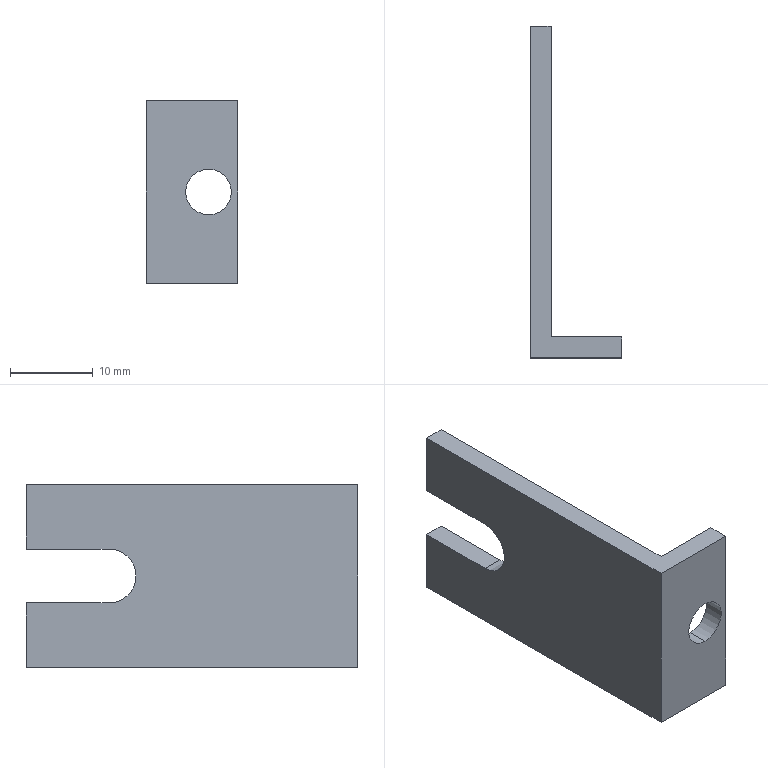Part | STEP file | slingshot track fixed block | 1 solid | 14 faces | box 11 x 40 x 22 mm | volume 2404 mm3 | plane 11 | cylinder 3 | commonest cylinder face diameters 5.5 x2 6.5 x1
STEP:
#1=CARTESIAN_POINT('',(0.,0.,0.));
#2=DIRECTION('',(0.,0.,1.));
#3=DIRECTION('',(1.,0.,0.));
#4=AXIS2_PLACEMENT_3D('',#1,#2,#3);
#5=CARTESIAN_POINT('',(7.5,0.,13.75));
#6=VERTEX_POINT('',#5);
#7=CARTESIAN_POINT('',(7.5,2.5,13.75));
#8=VERTEX_POINT('',#7);
#9=CARTESIAN_POINT('',(7.5,-19.5,13.75));
#10=DIRECTION('',(0.,1.,0.));
#11=VECTOR('',#10,1.);
#12=LINE('',#9,#11);
#13=CARTESIAN_POINT('',(7.5,-19.5,11.));
#14=DIRECTION('',(0.,1.,0.));
#15=DIRECTION('',(0.,0.,1.));
#16=AXIS2_PLACEMENT_3D('',#13,#14,#15);
#17=CYLINDRICAL_SURFACE('',#16,2.75);
#18=CARTESIAN_POINT('',(6.283,0.));
#19=DIRECTION('',(0.,1.));
#20=VECTOR('',#19,1.);
#21=LINE('',#18,#20);
#22=(GEOMETRIC_REPRESENTATION_CONTEXT(2)PARAMETRIC_REPRESENTATION_CONTEXT()REPRESENTATION_CONTEXT('',''));
#23=DEFINITIONAL_REPRESENTATION('',(#21),#22);
#24=PCURVE('',#17,#23);
#25=CARTESIAN_POINT('',(7.5,-19.5,11.));
#26=DIRECTION('',(0.,1.,0.));
#27=DIRECTION('',(0.,0.,1.));
#28=AXIS2_PLACEMENT_3D('',#25,#26,#27);
#29=CYLINDRICAL_SURFACE('',#28,2.75);
#30=CARTESIAN_POINT('',(0.,0.));
#31=DIRECTION('',(0.,1.));
#32=VECTOR('',#31,1.);
#33=LINE('',#30,#32);
#34=(GEOMETRIC_REPRESENTATION_CONTEXT(2)PARAMETRIC_REPRESENTATION_CONTEXT()REPRESENTATION_CONTEXT('',''));
#35=DEFINITIONAL_REPRESENTATION('',(#33),#34);
#36=PCURVE('',#29,#35);
#37=SURFACE_CURVE('',#12,(#24,#36),.PCURVE_S1.);
#38=EDGE_CURVE('',#6,#8,#37,.T.);
#39=ORIENTED_EDGE('',*,*,#38,.T.);
#40=CARTESIAN_POINT('',(7.5,2.5,8.25));
#41=VERTEX_POINT('',#40);
#42=CARTESIAN_POINT('',(7.5,2.5,11.));
#43=DIRECTION('',(0.,1.,0.));
#44=DIRECTION('',(0.,0.,1.));
#45=AXIS2_PLACEMENT_3D('',#42,#43,#44);
#46=CIRCLE('',#45,2.75);
#47=CARTESIAN_POINT('',(0.,22.));
#48=DIRECTION('',(1.,0.));
#49=VECTOR('',#48,1.);
#50=LINE('',#47,#49);
#51=(GEOMETRIC_REPRESENTATION_CONTEXT(2)PARAMETRIC_REPRESENTATION_CONTEXT()REPRESENTATION_CONTEXT('',''));
#52=DEFINITIONAL_REPRESENTATION('',(#50),#51);
#53=PCURVE('',#17,#52);
#54=CARTESIAN_POINT('',(2.5,2.5,22.));
#55=DIRECTION('',(0.,-1.,0.));
#56=DIRECTION('',(0.,0.,-1.));
#57=AXIS2_PLACEMENT_3D('',#54,#55,#56);
#58=PLANE('',#57);
#59=CARTESIAN_POINT('',(8.25,5.));
#60=CARTESIAN_POINT('',(8.25,9.763));
#61=CARTESIAN_POINT('',(12.375,7.382));
#62=CARTESIAN_POINT('',(16.5,5.));
#63=CARTESIAN_POINT('',(12.375,2.618));
#64=CARTESIAN_POINT('',(8.25,0.2369));
#65=CARTESIAN_POINT('',(8.25,5.));
#66=(BOUNDED_CURVE()B_SPLINE_CURVE(2,(#59,#60,#61,#62,#63,#64,#65),.UNSPECIFIED.,.T.,.F.)B_SPLINE_CURVE_WITH_KNOTS((1,2,2,2,2,1),(-2.094,0.,2.094,4.189,6.283,8.378),.UNSPECIFIED.)CURVE()GEOMETRIC_REPRESENTATION_ITEM()RATIONAL_B_SPLINE_CURVE((1.,0.5,1.,0.5,1.,0.5,1.))REPRESENTATION_ITEM(''));
#67=(GEOMETRIC_REPRESENTATION_CONTEXT(2)PARAMETRIC_REPRESENTATION_CONTEXT()REPRESENTATION_CONTEXT('',''));
#68=DEFINITIONAL_REPRESENTATION('',(#66),#67);
#69=PCURVE('',#58,#68);
#70=SURFACE_CURVE('',#46,(#53,#69),.PCURVE_S1.);
#71=EDGE_CURVE('',#41,#8,#70,.T.);
#72=ORIENTED_EDGE('',*,*,#71,.F.);
#73=CARTESIAN_POINT('',(7.5,0.,8.25));
#74=VERTEX_POINT('',#73);
#75=CARTESIAN_POINT('',(7.5,-19.5,8.25));
#76=DIRECTION('',(0.,1.,0.));
#77=VECTOR('',#76,1.);
#78=LINE('',#75,#77);
#79=CARTESIAN_POINT('',(3.142,0.));
#80=DIRECTION('',(0.,1.));
#81=VECTOR('',#80,1.);
#82=LINE('',#79,#81);
#83=(GEOMETRIC_REPRESENTATION_CONTEXT(2)PARAMETRIC_REPRESENTATION_CONTEXT()REPRESENTATION_CONTEXT('',''));
#84=DEFINITIONAL_REPRESENTATION('',(#82),#83);
#85=PCURVE('',#17,#84);
#86=CARTESIAN_POINT('',(3.142,0.));
#87=DIRECTION('',(0.,1.));
#88=VECTOR('',#87,1.);
#89=LINE('',#86,#88);
#90=(GEOMETRIC_REPRESENTATION_CONTEXT(2)PARAMETRIC_REPRESENTATION_CONTEXT()REPRESENTATION_CONTEXT('',''));
#91=DEFINITIONAL_REPRESENTATION('',(#89),#90);
#92=PCURVE('',#29,#91);
#93=SURFACE_CURVE('',#78,(#85,#92),.PCURVE_S1.);
#94=EDGE_CURVE('',#74,#41,#93,.T.);
#95=ORIENTED_EDGE('',*,*,#94,.F.);
#96=CARTESIAN_POINT('',(7.5,0.,11.));
#97=DIRECTION('',(0.,1.,0.));
#98=DIRECTION('',(0.,0.,1.));
#99=AXIS2_PLACEMENT_3D('',#96,#97,#98);
#100=CIRCLE('',#99,2.75);
#101=CARTESIAN_POINT('',(0.,19.5));
#102=DIRECTION('',(1.,0.));
#103=VECTOR('',#102,1.);
#104=LINE('',#101,#103);
#105=(GEOMETRIC_REPRESENTATION_CONTEXT(2)PARAMETRIC_REPRESENTATION_CONTEXT()REPRESENTATION_CONTEXT('',''));
#106=DEFINITIONAL_REPRESENTATION('',(#104),#105);
#107=PCURVE('',#17,#106);
#108=CARTESIAN_POINT('',(0.,0.,22.));
#109=DIRECTION('',(0.,1.,0.));
#110=DIRECTION('',(0.,0.,1.));
#111=AXIS2_PLACEMENT_3D('',#108,#109,#110);
#112=PLANE('',#111);
#113=CARTESIAN_POINT('',(-11.,7.5));
#114=DIRECTION('',(1.,0.));
#115=AXIS2_PLACEMENT_2D('',#113,#114);
#116=CIRCLE('',#115,2.75);
#117=(GEOMETRIC_REPRESENTATION_CONTEXT(2)PARAMETRIC_REPRESENTATION_CONTEXT()REPRESENTATION_CONTEXT('',''));
#118=DEFINITIONAL_REPRESENTATION('',(#116),#117);
#119=PCURVE('',#112,#118);
#120=SURFACE_CURVE('',#100,(#107,#119),.PCURVE_S1.);
#121=EDGE_CURVE('',#74,#6,#120,.T.);
#122=ORIENTED_EDGE('',*,*,#121,.T.);
#123=EDGE_LOOP('',(#39,#72,#95,#122));
#124=FACE_BOUND('',#123,.F.);
#125=ADVANCED_FACE('',(#124),#17,.F.);
#126=CARTESIAN_POINT('',(0.,40.,7.75));
#127=VERTEX_POINT('',#126);
#128=CARTESIAN_POINT('',(0.,40.,0.));
#129=VERTEX_POINT('',#128);
#130=CARTESIAN_POINT('',(0.,40.,22.));
#131=DIRECTION('',(0.,0.,-1.));
#132=VECTOR('',#131,1.);
#133=LINE('',#130,#132);
#134=CARTESIAN_POINT('',(0.,40.,22.));
#135=DIRECTION('',(0.,-1.,0.));
#136=DIRECTION('',(0.,0.,-1.));
#137=AXIS2_PLACEMENT_3D('',#134,#135,#136);
#138=PLANE('',#137);
#139=CARTESIAN_POINT('',(0.,0.));
#140=DIRECTION('',(1.,0.));
#141=VECTOR('',#140,1.);
#142=LINE('',#139,#141);
#143=(GEOMETRIC_REPRESENTATION_CONTEXT(2)PARAMETRIC_REPRESENTATION_CONTEXT()REPRESENTATION_CONTEXT('',''));
#144=DEFINITIONAL_REPRESENTATION('',(#142),#143);
#145=PCURVE('',#138,#144);
#146=CARTESIAN_POINT('',(0.,0.,22.));
#147=DIRECTION('',(1.,0.,0.));
#148=DIRECTION('',(0.,0.,-1.));
#149=AXIS2_PLACEMENT_3D('',#146,#147,#148);
#150=PLANE('',#149);
#151=CARTESIAN_POINT('',(0.,40.));
#152=DIRECTION('',(1.,0.));
#153=VECTOR('',#152,1.);
#154=LINE('',#151,#153);
#155=(GEOMETRIC_REPRESENTATION_CONTEXT(2)PARAMETRIC_REPRESENTATION_CONTEXT()REPRESENTATION_CONTEXT('',''));
#156=DEFINITIONAL_REPRESENTATION('',(#154),#155);
#157=PCURVE('',#150,#156);
#158=SURFACE_CURVE('',#133,(#145,#157),.PCURVE_S1.);
#159=EDGE_CURVE('',#127,#129,#158,.T.);
#160=ORIENTED_EDGE('',*,*,#159,.F.);
#161=CARTESIAN_POINT('',(2.5,40.,7.75));
#162=VERTEX_POINT('',#161);
#163=CARTESIAN_POINT('',(0.,40.,7.75));
#164=DIRECTION('',(1.,0.,0.));
#165=VECTOR('',#164,1.);
#166=LINE('',#163,#165);
#167=CARTESIAN_POINT('',(14.25,0.));
#168=DIRECTION('',(0.,1.));
#169=VECTOR('',#168,1.);
#170=LINE('',#167,#169);
#171=(GEOMETRIC_REPRESENTATION_CONTEXT(2)PARAMETRIC_REPRESENTATION_CONTEXT()REPRESENTATION_CONTEXT('',''));
#172=DEFINITIONAL_REPRESENTATION('',(#170),#171);
#173=PCURVE('',#138,#172);
#174=CARTESIAN_POINT('',(22.,30.,7.75));
#175=DIRECTION('',(0.,0.,-1.));
#176=DIRECTION('',(-1.,0.,0.));
#177=AXIS2_PLACEMENT_3D('',#174,#175,#176);
#178=PLANE('',#177);
#179=CARTESIAN_POINT('',(22.,10.));
#180=DIRECTION('',(-1.,0.));
#181=VECTOR('',#180,1.);
#182=LINE('',#179,#181);
#183=(GEOMETRIC_REPRESENTATION_CONTEXT(2)PARAMETRIC_REPRESENTATION_CONTEXT()REPRESENTATION_CONTEXT('',''));
#184=DEFINITIONAL_REPRESENTATION('',(#182),#183);
#185=PCURVE('',#178,#184);
#186=SURFACE_CURVE('',#166,(#173,#185),.PCURVE_S1.);
#187=EDGE_CURVE('',#127,#162,#186,.T.);
#188=ORIENTED_EDGE('',*,*,#187,.T.);
#189=CARTESIAN_POINT('',(2.5,40.,0.));
#190=VERTEX_POINT('',#189);
#191=CARTESIAN_POINT('',(2.5,40.,22.));
#192=DIRECTION('',(0.,0.,-1.));
#193=VECTOR('',#192,1.);
#194=LINE('',#191,#193);
#195=CARTESIAN_POINT('',(0.,2.5));
#196=DIRECTION('',(1.,0.));
#197=VECTOR('',#196,1.);
#198=LINE('',#195,#197);
#199=(GEOMETRIC_REPRESENTATION_CONTEXT(2)PARAMETRIC_REPRESENTATION_CONTEXT()REPRESENTATION_CONTEXT('',''));
#200=DEFINITIONAL_REPRESENTATION('',(#198),#199);
#201=PCURVE('',#138,#200);
#202=CARTESIAN_POINT('',(2.5,2.5,22.));
#203=DIRECTION('',(-1.,0.,0.));
#204=DIRECTION('',(0.,-1.,0.));
#205=AXIS2_PLACEMENT_3D('',#202,#203,#204);
#206=PLANE('',#205);
#207=CARTESIAN_POINT('',(-37.5,0.));
#208=DIRECTION('',(0.,-1.));
#209=VECTOR('',#208,1.);
#210=LINE('',#207,#209);
#211=(GEOMETRIC_REPRESENTATION_CONTEXT(2)PARAMETRIC_REPRESENTATION_CONTEXT()REPRESENTATION_CONTEXT('',''));
#212=DEFINITIONAL_REPRESENTATION('',(#210),#211);
#213=PCURVE('',#206,#212);
#214=SURFACE_CURVE('',#194,(#201,#213),.PCURVE_S1.);
#215=EDGE_CURVE('',#162,#190,#214,.T.);
#216=ORIENTED_EDGE('',*,*,#215,.T.);
#217=CARTESIAN_POINT('',(0.,40.,0.));
#218=DIRECTION('',(-1.,0.,0.));
#219=VECTOR('',#218,1.);
#220=LINE('',#217,#219);
#221=CARTESIAN_POINT('',(22.,0.));
#222=DIRECTION('',(0.,-1.));
#223=VECTOR('',#222,1.);
#224=LINE('',#221,#223);
#225=(GEOMETRIC_REPRESENTATION_CONTEXT(2)PARAMETRIC_REPRESENTATION_CONTEXT()REPRESENTATION_CONTEXT('',''));
#226=DEFINITIONAL_REPRESENTATION('',(#224),#225);
#227=PCURVE('',#138,#226);
#228=CARTESIAN_POINT('',(0.,40.,0.));
#229=DIRECTION('',(0.,0.,-1.));
#230=DIRECTION('',(-1.,0.,0.));
#231=AXIS2_PLACEMENT_3D('',#228,#229,#230);
#232=PLANE('',#231);
#233=CARTESIAN_POINT('',(0.,0.));
#234=DIRECTION('',(1.,0.));
#235=VECTOR('',#234,1.);
#236=LINE('',#233,#235);
#237=(GEOMETRIC_REPRESENTATION_CONTEXT(2)PARAMETRIC_REPRESENTATION_CONTEXT()REPRESENTATION_CONTEXT('',''));
#238=DEFINITIONAL_REPRESENTATION('',(#236),#237);
#239=PCURVE('',#232,#238);
#240=SURFACE_CURVE('',#220,(#227,#239),.PCURVE_S1.);
#241=EDGE_CURVE('',#190,#129,#240,.T.);
#242=ORIENTED_EDGE('',*,*,#241,.T.);
#243=EDGE_LOOP('',(#160,#188,#216,#242));
#244=FACE_BOUND('',#243,.T.);
#245=ADVANCED_FACE('',(#244),#138,.F.);
#246=CARTESIAN_POINT('',(0.,30.,7.75));
#247=VERTEX_POINT('',#246);
#248=CARTESIAN_POINT('',(0.,30.,14.25));
#249=VERTEX_POINT('',#248);
#250=CARTESIAN_POINT('',(0.,30.,11.));
#251=DIRECTION('',(-1.,0.,0.));
#252=DIRECTION('',(0.,0.,1.));
#253=AXIS2_PLACEMENT_3D('',#250,#251,#252);
#254=CIRCLE('',#253,3.25);
#255=CARTESIAN_POINT('',(7.75,30.));
#256=CARTESIAN_POINT('',(7.75,35.629));
#257=CARTESIAN_POINT('',(12.625,32.815));
#258=CARTESIAN_POINT('',(17.5,30.));
#259=CARTESIAN_POINT('',(12.625,27.185));
#260=CARTESIAN_POINT('',(7.75,24.371));
#261=CARTESIAN_POINT('',(7.75,30.));
#262=(BOUNDED_CURVE()B_SPLINE_CURVE(2,(#255,#256,#257,#258,#259,#260,#261),.UNSPECIFIED.,.T.,.F.)B_SPLINE_CURVE_WITH_KNOTS((1,2,2,2,2,1),(-2.094,0.,2.094,4.189,6.283,8.378),.UNSPECIFIED.)CURVE()GEOMETRIC_REPRESENTATION_ITEM()RATIONAL_B_SPLINE_CURVE((1.,0.5,1.,0.5,1.,0.5,1.))REPRESENTATION_ITEM(''));
#263=(GEOMETRIC_REPRESENTATION_CONTEXT(2)PARAMETRIC_REPRESENTATION_CONTEXT()REPRESENTATION_CONTEXT('',''));
#264=DEFINITIONAL_REPRESENTATION('',(#262),#263);
#265=PCURVE('',#150,#264);
#266=CARTESIAN_POINT('',(22.,30.,11.));
#267=DIRECTION('',(-1.,0.,0.));
#268=DIRECTION('',(0.,0.,1.));
#269=AXIS2_PLACEMENT_3D('',#266,#267,#268);
#270=CYLINDRICAL_SURFACE('',#269,3.25);
#271=CARTESIAN_POINT('',(0.,22.));
#272=DIRECTION('',(1.,0.));
#273=VECTOR('',#272,1.);
#274=LINE('',#271,#273);
#275=(GEOMETRIC_REPRESENTATION_CONTEXT(2)PARAMETRIC_REPRESENTATION_CONTEXT()REPRESENTATION_CONTEXT('',''));
#276=DEFINITIONAL_REPRESENTATION('',(#274),#275);
#277=PCURVE('',#270,#276);
#278=SURFACE_CURVE('',#254,(#265,#277),.PCURVE_S1.);
#279=EDGE_CURVE('',#247,#249,#278,.T.);
#280=ORIENTED_EDGE('',*,*,#279,.F.);
#281=CARTESIAN_POINT('',(0.,30.,7.75));
#282=DIRECTION('',(0.,-1.,0.));
#283=VECTOR('',#282,1.);
#284=LINE('',#281,#283);
#285=CARTESIAN_POINT('',(14.25,30.));
#286=DIRECTION('',(0.,-1.));
#287=VECTOR('',#286,1.);
#288=LINE('',#285,#287);
#289=(GEOMETRIC_REPRESENTATION_CONTEXT(2)PARAMETRIC_REPRESENTATION_CONTEXT()REPRESENTATION_CONTEXT('',''));
#290=DEFINITIONAL_REPRESENTATION('',(#288),#289);
#291=PCURVE('',#150,#290);
#292=CARTESIAN_POINT('',(22.,0.));
#293=DIRECTION('',(0.,-1.));
#294=VECTOR('',#293,1.);
#295=LINE('',#292,#294);
#296=(GEOMETRIC_REPRESENTATION_CONTEXT(2)PARAMETRIC_REPRESENTATION_CONTEXT()REPRESENTATION_CONTEXT('',''));
#297=DEFINITIONAL_REPRESENTATION('',(#295),#296);
#298=PCURVE('',#178,#297);
#299=SURFACE_CURVE('',#284,(#291,#298),.PCURVE_S1.);
#300=EDGE_CURVE('',#127,#247,#299,.T.);
#301=ORIENTED_EDGE('',*,*,#300,.F.);
#302=ORIENTED_EDGE('',*,*,#159,.T.);
#303=CARTESIAN_POINT('',(0.,0.,0.));
#304=VERTEX_POINT('',#303);
#305=CARTESIAN_POINT('',(0.,0.,0.));
#306=DIRECTION('',(0.,-1.,0.));
#307=VECTOR('',#306,1.);
#308=LINE('',#305,#307);
#309=CARTESIAN_POINT('',(22.,0.));
#310=DIRECTION('',(0.,-1.));
#311=VECTOR('',#310,1.);
#312=LINE('',#309,#311);
#313=(GEOMETRIC_REPRESENTATION_CONTEXT(2)PARAMETRIC_REPRESENTATION_CONTEXT()REPRESENTATION_CONTEXT('',''));
#314=DEFINITIONAL_REPRESENTATION('',(#312),#313);
#315=PCURVE('',#150,#314);
#316=CARTESIAN_POINT('',(0.,-40.));
#317=DIRECTION('',(0.,-1.));
#318=VECTOR('',#317,1.);
#319=LINE('',#316,#318);
#320=(GEOMETRIC_REPRESENTATION_CONTEXT(2)PARAMETRIC_REPRESENTATION_CONTEXT()REPRESENTATION_CONTEXT('',''));
#321=DEFINITIONAL_REPRESENTATION('',(#319),#320);
#322=PCURVE('',#232,#321);
#323=SURFACE_CURVE('',#308,(#315,#322),.PCURVE_S1.);
#324=EDGE_CURVE('',#129,#304,#323,.T.);
#325=ORIENTED_EDGE('',*,*,#324,.T.);
#326=CARTESIAN_POINT('',(0.,0.,22.));
#327=VERTEX_POINT('',#326);
#328=CARTESIAN_POINT('',(0.,0.,22.));
#329=DIRECTION('',(0.,0.,-1.));
#330=VECTOR('',#329,1.);
#331=LINE('',#328,#330);
#332=CARTESIAN_POINT('',(0.,0.));
#333=DIRECTION('',(1.,0.));
#334=VECTOR('',#333,1.);
#335=LINE('',#332,#334);
#336=(GEOMETRIC_REPRESENTATION_CONTEXT(2)PARAMETRIC_REPRESENTATION_CONTEXT()REPRESENTATION_CONTEXT('',''));
#337=DEFINITIONAL_REPRESENTATION('',(#335),#336);
#338=PCURVE('',#150,#337);
#339=CARTESIAN_POINT('',(0.,0.));
#340=DIRECTION('',(-1.,0.));
#341=VECTOR('',#340,1.);
#342=LINE('',#339,#341);
#343=(GEOMETRIC_REPRESENTATION_CONTEXT(2)PARAMETRIC_REPRESENTATION_CONTEXT()REPRESENTATION_CONTEXT('',''));
#344=DEFINITIONAL_REPRESENTATION('',(#342),#343);
#345=PCURVE('',#112,#344);
#346=SURFACE_CURVE('',#331,(#338,#345),.PCURVE_S1.);
#347=EDGE_CURVE('',#327,#304,#346,.T.);
#348=ORIENTED_EDGE('',*,*,#347,.F.);
#349=CARTESIAN_POINT('',(0.,40.,22.));
#350=VERTEX_POINT('',#349);
#351=CARTESIAN_POINT('',(0.,0.,22.));
#352=DIRECTION('',(0.,-1.,0.));
#353=VECTOR('',#352,1.);
#354=LINE('',#351,#353);
#355=CARTESIAN_POINT('',(0.,0.));
#356=DIRECTION('',(0.,-1.));
#357=VECTOR('',#356,1.);
#358=LINE('',#355,#357);
#359=(GEOMETRIC_REPRESENTATION_CONTEXT(2)PARAMETRIC_REPRESENTATION_CONTEXT()REPRESENTATION_CONTEXT('',''));
#360=DEFINITIONAL_REPRESENTATION('',(#358),#359);
#361=PCURVE('',#150,#360);
#362=CARTESIAN_POINT('',(0.,40.,22.));
#363=DIRECTION('',(0.,0.,-1.));
#364=DIRECTION('',(-1.,0.,0.));
#365=AXIS2_PLACEMENT_3D('',#362,#363,#364);
#366=PLANE('',#365);
#367=CARTESIAN_POINT('',(0.,-40.));
#368=DIRECTION('',(0.,-1.));
#369=VECTOR('',#368,1.);
#370=LINE('',#367,#369);
#371=(GEOMETRIC_REPRESENTATION_CONTEXT(2)PARAMETRIC_REPRESENTATION_CONTEXT()REPRESENTATION_CONTEXT('',''));
#372=DEFINITIONAL_REPRESENTATION('',(#370),#371);
#373=PCURVE('',#366,#372);
#374=SURFACE_CURVE('',#354,(#361,#373),.PCURVE_S1.);
#375=EDGE_CURVE('',#350,#327,#374,.T.);
#376=ORIENTED_EDGE('',*,*,#375,.F.);
#377=CARTESIAN_POINT('',(0.,40.,14.25));
#378=VERTEX_POINT('',#377);
#379=CARTESIAN_POINT('',(0.,40.,22.));
#380=DIRECTION('',(0.,0.,-1.));
#381=VECTOR('',#380,1.);
#382=LINE('',#379,#381);
#383=CARTESIAN_POINT('',(0.,40.));
#384=DIRECTION('',(1.,0.));
#385=VECTOR('',#384,1.);
#386=LINE('',#383,#385);
#387=(GEOMETRIC_REPRESENTATION_CONTEXT(2)PARAMETRIC_REPRESENTATION_CONTEXT()REPRESENTATION_CONTEXT('',''));
#388=DEFINITIONAL_REPRESENTATION('',(#386),#387);
#389=PCURVE('',#150,#388);
#390=CARTESIAN_POINT('',(0.,40.,22.));
#391=DIRECTION('',(0.,-1.,0.));
#392=DIRECTION('',(0.,0.,-1.));
#393=AXIS2_PLACEMENT_3D('',#390,#391,#392);
#394=PLANE('',#393);
#395=CARTESIAN_POINT('',(0.,0.));
#396=DIRECTION('',(1.,0.));
#397=VECTOR('',#396,1.);
#398=LINE('',#395,#397);
#399=(GEOMETRIC_REPRESENTATION_CONTEXT(2)PARAMETRIC_REPRESENTATION_CONTEXT()REPRESENTATION_CONTEXT('',''));
#400=DEFINITIONAL_REPRESENTATION('',(#398),#399);
#401=PCURVE('',#394,#400);
#402=SURFACE_CURVE('',#382,(#389,#401),.PCURVE_S1.);
#403=EDGE_CURVE('',#350,#378,#402,.T.);
#404=ORIENTED_EDGE('',*,*,#403,.T.);
#405=CARTESIAN_POINT('',(0.,30.,14.25));
#406=DIRECTION('',(0.,1.,0.));
#407=VECTOR('',#406,1.);
#408=LINE('',#405,#407);
#409=CARTESIAN_POINT('',(7.75,30.));
#410=DIRECTION('',(0.,1.));
#411=VECTOR('',#410,1.);
#412=LINE('',#409,#411);
#413=(GEOMETRIC_REPRESENTATION_CONTEXT(2)PARAMETRIC_REPRESENTATION_CONTEXT()REPRESENTATION_CONTEXT('',''));
#414=DEFINITIONAL_REPRESENTATION('',(#412),#413);
#415=PCURVE('',#150,#414);
#416=CARTESIAN_POINT('',(22.,30.,14.25));
#417=DIRECTION('',(0.,0.,1.));
#418=DIRECTION('',(1.,0.,0.));
#419=AXIS2_PLACEMENT_3D('',#416,#417,#418);
#420=PLANE('',#419);
#421=CARTESIAN_POINT('',(-22.,0.));
#422=DIRECTION('',(0.,1.));
#423=VECTOR('',#422,1.);
#424=LINE('',#421,#423);
#425=(GEOMETRIC_REPRESENTATION_CONTEXT(2)PARAMETRIC_REPRESENTATION_CONTEXT()REPRESENTATION_CONTEXT('',''));
#426=DEFINITIONAL_REPRESENTATION('',(#424),#425);
#427=PCURVE('',#420,#426);
#428=SURFACE_CURVE('',#408,(#415,#427),.PCURVE_S1.);
#429=EDGE_CURVE('',#249,#378,#428,.T.);
#430=ORIENTED_EDGE('',*,*,#429,.F.);
#431=EDGE_LOOP('',(#280,#301,#302,#325,#348,#376,#404,#430));
#432=FACE_BOUND('',#431,.T.);
#433=ADVANCED_FACE('',(#432),#150,.F.);
#434=CARTESIAN_POINT('',(7.5,0.,11.));
#435=DIRECTION('',(0.,1.,0.));
#436=DIRECTION('',(0.,0.,1.));
#437=AXIS2_PLACEMENT_3D('',#434,#435,#436);
#438=CIRCLE('',#437,2.75);
#439=CARTESIAN_POINT('',(-11.,7.5));
#440=DIRECTION('',(1.,0.));
#441=AXIS2_PLACEMENT_2D('',#439,#440);
#442=CIRCLE('',#441,2.75);
#443=(GEOMETRIC_REPRESENTATION_CONTEXT(2)PARAMETRIC_REPRESENTATION_CONTEXT()REPRESENTATION_CONTEXT('',''));
#444=DEFINITIONAL_REPRESENTATION('',(#442),#443);
#445=PCURVE('',#112,#444);
#446=CARTESIAN_POINT('',(0.,19.5));
#447=DIRECTION('',(1.,0.));
#448=VECTOR('',#447,1.);
#449=LINE('',#446,#448);
#450=(GEOMETRIC_REPRESENTATION_CONTEXT(2)PARAMETRIC_REPRESENTATION_CONTEXT()REPRESENTATION_CONTEXT('',''));
#451=DEFINITIONAL_REPRESENTATION('',(#449),#450);
#452=PCURVE('',#29,#451);
#453=SURFACE_CURVE('',#438,(#445,#452),.PCURVE_S1.);
#454=EDGE_CURVE('',#6,#74,#453,.T.);
#455=ORIENTED_EDGE('',*,*,#454,.T.);
#456=ORIENTED_EDGE('',*,*,#121,.T.);
#457=EDGE_LOOP('',(#455,#456));
#458=FACE_BOUND('',#457,.T.);
#459=CARTESIAN_POINT('',(11.,0.,0.));
#460=VERTEX_POINT('',#459);
#461=CARTESIAN_POINT('',(0.,0.,0.));
#462=DIRECTION('',(1.,0.,0.));
#463=VECTOR('',#462,1.);
#464=LINE('',#461,#463);
#465=CARTESIAN_POINT('',(-22.,0.));
#466=DIRECTION('',(0.,1.));
#467=VECTOR('',#466,1.);
#468=LINE('',#465,#467);
#469=(GEOMETRIC_REPRESENTATION_CONTEXT(2)PARAMETRIC_REPRESENTATION_CONTEXT()REPRESENTATION_CONTEXT('',''));
#470=DEFINITIONAL_REPRESENTATION('',(#468),#469);
#471=PCURVE('',#112,#470);
#472=CARTESIAN_POINT('',(0.,-40.));
#473=DIRECTION('',(-1.,0.));
#474=VECTOR('',#473,1.);
#475=LINE('',#472,#474);
#476=(GEOMETRIC_REPRESENTATION_CONTEXT(2)PARAMETRIC_REPRESENTATION_CONTEXT()REPRESENTATION_CONTEXT('',''));
#477=DEFINITIONAL_REPRESENTATION('',(#475),#476);
#478=PCURVE('',#232,#477);
#479=SURFACE_CURVE('',#464,(#471,#478),.PCURVE_S1.);
#480=EDGE_CURVE('',#304,#460,#479,.T.);
#481=ORIENTED_EDGE('',*,*,#480,.T.);
#482=CARTESIAN_POINT('',(11.,0.,22.));
#483=VERTEX_POINT('',#482);
#484=CARTESIAN_POINT('',(11.,0.,22.));
#485=DIRECTION('',(0.,0.,-1.));
#486=VECTOR('',#485,1.);
#487=LINE('',#484,#486);
#488=CARTESIAN_POINT('',(0.,11.));
#489=DIRECTION('',(-1.,0.));
#490=VECTOR('',#489,1.);
#491=LINE('',#488,#490);
#492=(GEOMETRIC_REPRESENTATION_CONTEXT(2)PARAMETRIC_REPRESENTATION_CONTEXT()REPRESENTATION_CONTEXT('',''));
#493=DEFINITIONAL_REPRESENTATION('',(#491),#492);
#494=PCURVE('',#112,#493);
#495=CARTESIAN_POINT('',(11.,0.,22.));
#496=DIRECTION('',(-1.,0.,0.));
#497=DIRECTION('',(0.,0.,1.));
#498=AXIS2_PLACEMENT_3D('',#495,#496,#497);
#499=PLANE('',#498);
#500=CARTESIAN_POINT('',(0.,0.));
#501=DIRECTION('',(-1.,0.));
#502=VECTOR('',#501,1.);
#503=LINE('',#500,#502);
#504=(GEOMETRIC_REPRESENTATION_CONTEXT(2)PARAMETRIC_REPRESENTATION_CONTEXT()REPRESENTATION_CONTEXT('',''));
#505=DEFINITIONAL_REPRESENTATION('',(#503),#504);
#506=PCURVE('',#499,#505);
#507=SURFACE_CURVE('',#487,(#494,#506),.PCURVE_S1.);
#508=EDGE_CURVE('',#483,#460,#507,.T.);
#509=ORIENTED_EDGE('',*,*,#508,.F.);
#510=CARTESIAN_POINT('',(0.,0.,22.));
#511=DIRECTION('',(1.,0.,0.));
#512=VECTOR('',#511,1.);
#513=LINE('',#510,#512);
#514=CARTESIAN_POINT('',(0.,0.));
#515=DIRECTION('',(0.,1.));
#516=VECTOR('',#515,1.);
#517=LINE('',#514,#516);
#518=(GEOMETRIC_REPRESENTATION_CONTEXT(2)PARAMETRIC_REPRESENTATION_CONTEXT()REPRESENTATION_CONTEXT('',''));
#519=DEFINITIONAL_REPRESENTATION('',(#517),#518);
#520=PCURVE('',#112,#519);
#521=CARTESIAN_POINT('',(0.,-40.));
#522=DIRECTION('',(-1.,0.));
#523=VECTOR('',#522,1.);
#524=LINE('',#521,#523);
#525=(GEOMETRIC_REPRESENTATION_CONTEXT(2)PARAMETRIC_REPRESENTATION_CONTEXT()REPRESENTATION_CONTEXT('',''));
#526=DEFINITIONAL_REPRESENTATION('',(#524),#525);
#527=PCURVE('',#366,#526);
#528=SURFACE_CURVE('',#513,(#520,#527),.PCURVE_S1.);
#529=EDGE_CURVE('',#327,#483,#528,.T.);
#530=ORIENTED_EDGE('',*,*,#529,.F.);
#531=ORIENTED_EDGE('',*,*,#347,.T.);
#532=EDGE_LOOP('',(#481,#509,#530,#531));
#533=FACE_BOUND('',#532,.T.);
#534=ADVANCED_FACE('',(#458,#533),#112,.F.);
#535=CARTESIAN_POINT('',(11.,2.5,0.));
#536=VERTEX_POINT('',#535);
#537=CARTESIAN_POINT('',(11.,0.,0.));
#538=DIRECTION('',(0.,1.,0.));
#539=VECTOR('',#538,1.);
#540=LINE('',#537,#539);
#541=CARTESIAN_POINT('',(-22.,0.));
#542=DIRECTION('',(0.,1.));
#543=VECTOR('',#542,1.);
#544=LINE('',#541,#543);
#545=(GEOMETRIC_REPRESENTATION_CONTEXT(2)PARAMETRIC_REPRESENTATION_CONTEXT()REPRESENTATION_CONTEXT('',''));
#546=DEFINITIONAL_REPRESENTATION('',(#544),#545);
#547=PCURVE('',#499,#546);
#548=CARTESIAN_POINT('',(-11.,-40.));
#549=DIRECTION('',(0.,1.));
#550=VECTOR('',#549,1.);
#551=LINE('',#548,#550);
#552=(GEOMETRIC_REPRESENTATION_CONTEXT(2)PARAMETRIC_REPRESENTATION_CONTEXT()REPRESENTATION_CONTEXT('',''));
#553=DEFINITIONAL_REPRESENTATION('',(#551),#552);
#554=PCURVE('',#232,#553);
#555=SURFACE_CURVE('',#540,(#547,#554),.PCURVE_S1.);
#556=EDGE_CURVE('',#460,#536,#555,.T.);
#557=ORIENTED_EDGE('',*,*,#556,.T.);
#558=CARTESIAN_POINT('',(11.,2.5,22.));
#559=VERTEX_POINT('',#558);
#560=CARTESIAN_POINT('',(11.,2.5,22.));
#561=DIRECTION('',(0.,0.,-1.));
#562=VECTOR('',#561,1.);
#563=LINE('',#560,#562);
#564=CARTESIAN_POINT('',(0.,2.5));
#565=DIRECTION('',(-1.,0.));
#566=VECTOR('',#565,1.);
#567=LINE('',#564,#566);
#568=(GEOMETRIC_REPRESENTATION_CONTEXT(2)PARAMETRIC_REPRESENTATION_CONTEXT()REPRESENTATION_CONTEXT('',''));
#569=DEFINITIONAL_REPRESENTATION('',(#567),#568);
#570=PCURVE('',#499,#569);
#571=CARTESIAN_POINT('',(0.,8.5));
#572=DIRECTION('',(1.,0.));
#573=VECTOR('',#572,1.);
#574=LINE('',#571,#573);
#575=(GEOMETRIC_REPRESENTATION_CONTEXT(2)PARAMETRIC_REPRESENTATION_CONTEXT()REPRESENTATION_CONTEXT('',''));
#576=DEFINITIONAL_REPRESENTATION('',(#574),#575);
#577=PCURVE('',#58,#576);
#578=SURFACE_CURVE('',#563,(#570,#577),.PCURVE_S1.);
#579=EDGE_CURVE('',#559,#536,#578,.T.);
#580=ORIENTED_EDGE('',*,*,#579,.F.);
#581=CARTESIAN_POINT('',(11.,0.,22.));
#582=DIRECTION('',(0.,1.,0.));
#583=VECTOR('',#582,1.);
#584=LINE('',#581,#583);
#585=CARTESIAN_POINT('',(0.,0.));
#586=DIRECTION('',(0.,1.));
#587=VECTOR('',#586,1.);
#588=LINE('',#585,#587);
#589=(GEOMETRIC_REPRESENTATION_CONTEXT(2)PARAMETRIC_REPRESENTATION_CONTEXT()REPRESENTATION_CONTEXT('',''));
#590=DEFINITIONAL_REPRESENTATION('',(#588),#589);
#591=PCURVE('',#499,#590);
#592=CARTESIAN_POINT('',(-11.,-40.));
#593=DIRECTION('',(0.,1.));
#594=VECTOR('',#593,1.);
#595=LINE('',#592,#594);
#596=(GEOMETRIC_REPRESENTATION_CONTEXT(2)PARAMETRIC_REPRESENTATION_CONTEXT()REPRESENTATION_CONTEXT('',''));
#597=DEFINITIONAL_REPRESENTATION('',(#595),#596);
#598=PCURVE('',#366,#597);
#599=SURFACE_CURVE('',#584,(#591,#598),.PCURVE_S1.);
#600=EDGE_CURVE('',#483,#559,#599,.T.);
#601=ORIENTED_EDGE('',*,*,#600,.F.);
#602=ORIENTED_EDGE('',*,*,#508,.T.);
#603=EDGE_LOOP('',(#557,#580,#601,#602));
#604=FACE_BOUND('',#603,.T.);
#605=ADVANCED_FACE('',(#604),#499,.F.);
#606=CARTESIAN_POINT('',(7.5,2.5,11.));
#607=DIRECTION('',(0.,1.,0.));
#608=DIRECTION('',(0.,0.,1.));
#609=AXIS2_PLACEMENT_3D('',#606,#607,#608);
#610=CIRCLE('',#609,2.75);
#611=CARTESIAN_POINT('',(8.25,5.));
#612=CARTESIAN_POINT('',(8.25,9.763));
#613=CARTESIAN_POINT('',(12.375,7.382));
#614=CARTESIAN_POINT('',(16.5,5.));
#615=CARTESIAN_POINT('',(12.375,2.618));
#616=CARTESIAN_POINT('',(8.25,0.2369));
#617=CARTESIAN_POINT('',(8.25,5.));
#618=(BOUNDED_CURVE()B_SPLINE_CURVE(2,(#611,#612,#613,#614,#615,#616,#617),.UNSPECIFIED.,.T.,.F.)B_SPLINE_CURVE_WITH_KNOTS((1,2,2,2,2,1),(-2.094,0.,2.094,4.189,6.283,8.378),.UNSPECIFIED.)CURVE()GEOMETRIC_REPRESENTATION_ITEM()RATIONAL_B_SPLINE_CURVE((1.,0.5,1.,0.5,1.,0.5,1.))REPRESENTATION_ITEM(''));
#619=(GEOMETRIC_REPRESENTATION_CONTEXT(2)PARAMETRIC_REPRESENTATION_CONTEXT()REPRESENTATION_CONTEXT('',''));
#620=DEFINITIONAL_REPRESENTATION('',(#618),#619);
#621=PCURVE('',#58,#620);
#622=CARTESIAN_POINT('',(0.,22.));
#623=DIRECTION('',(1.,0.));
#624=VECTOR('',#623,1.);
#625=LINE('',#622,#624);
#626=(GEOMETRIC_REPRESENTATION_CONTEXT(2)PARAMETRIC_REPRESENTATION_CONTEXT()REPRESENTATION_CONTEXT('',''));
#627=DEFINITIONAL_REPRESENTATION('',(#625),#626);
#628=PCURVE('',#29,#627);
#629=SURFACE_CURVE('',#610,(#621,#628),.PCURVE_S1.);
#630=EDGE_CURVE('',#8,#41,#629,.T.);
#631=ORIENTED_EDGE('',*,*,#630,.F.);
#632=ORIENTED_EDGE('',*,*,#71,.F.);
#633=EDGE_LOOP('',(#631,#632));
#634=FACE_BOUND('',#633,.T.);
#635=CARTESIAN_POINT('',(2.5,2.5,0.));
#636=VERTEX_POINT('',#635);
#637=CARTESIAN_POINT('',(2.5,2.5,0.));
#638=DIRECTION('',(-1.,0.,0.));
#639=VECTOR('',#638,1.);
#640=LINE('',#637,#639);
#641=CARTESIAN_POINT('',(22.,0.));
#642=DIRECTION('',(0.,-1.));
#643=VECTOR('',#642,1.);
#644=LINE('',#641,#643);
#645=(GEOMETRIC_REPRESENTATION_CONTEXT(2)PARAMETRIC_REPRESENTATION_CONTEXT()REPRESENTATION_CONTEXT('',''));
#646=DEFINITIONAL_REPRESENTATION('',(#644),#645);
#647=PCURVE('',#58,#646);
#648=CARTESIAN_POINT('',(-2.5,-37.5));
#649=DIRECTION('',(1.,0.));
#650=VECTOR('',#649,1.);
#651=LINE('',#648,#650);
#652=(GEOMETRIC_REPRESENTATION_CONTEXT(2)PARAMETRIC_REPRESENTATION_CONTEXT()REPRESENTATION_CONTEXT('',''));
#653=DEFINITIONAL_REPRESENTATION('',(#651),#652);
#654=PCURVE('',#232,#653);
#655=SURFACE_CURVE('',#640,(#647,#654),.PCURVE_S1.);
#656=EDGE_CURVE('',#536,#636,#655,.T.);
#657=ORIENTED_EDGE('',*,*,#656,.T.);
#658=CARTESIAN_POINT('',(2.5,2.5,22.));
#659=VERTEX_POINT('',#658);
#660=CARTESIAN_POINT('',(2.5,2.5,22.));
#661=DIRECTION('',(0.,0.,-1.));
#662=VECTOR('',#661,1.);
#663=LINE('',#660,#662);
#664=CARTESIAN_POINT('',(0.,0.));
#665=DIRECTION('',(1.,0.));
#666=VECTOR('',#665,1.);
#667=LINE('',#664,#666);
#668=(GEOMETRIC_REPRESENTATION_CONTEXT(2)PARAMETRIC_REPRESENTATION_CONTEXT()REPRESENTATION_CONTEXT('',''));
#669=DEFINITIONAL_REPRESENTATION('',(#667),#668);
#670=PCURVE('',#58,#669);
#671=CARTESIAN_POINT('',(0.,0.));
#672=DIRECTION('',(0.,-1.));
#673=VECTOR('',#672,1.);
#674=LINE('',#671,#673);
#675=(GEOMETRIC_REPRESENTATION_CONTEXT(2)PARAMETRIC_REPRESENTATION_CONTEXT()REPRESENTATION_CONTEXT('',''));
#676=DEFINITIONAL_REPRESENTATION('',(#674),#675);
#677=PCURVE('',#206,#676);
#678=SURFACE_CURVE('',#663,(#670,#677),.PCURVE_S1.);
#679=EDGE_CURVE('',#659,#636,#678,.T.);
#680=ORIENTED_EDGE('',*,*,#679,.F.);
#681=CARTESIAN_POINT('',(2.5,2.5,22.));
#682=DIRECTION('',(-1.,0.,0.));
#683=VECTOR('',#682,1.);
#684=LINE('',#681,#683);
#685=CARTESIAN_POINT('',(0.,0.));
#686=DIRECTION('',(0.,-1.));
#687=VECTOR('',#686,1.);
#688=LINE('',#685,#687);
#689=(GEOMETRIC_REPRESENTATION_CONTEXT(2)PARAMETRIC_REPRESENTATION_CONTEXT()REPRESENTATION_CONTEXT('',''));
#690=DEFINITIONAL_REPRESENTATION('',(#688),#689);
#691=PCURVE('',#58,#690);
#692=CARTESIAN_POINT('',(-2.5,-37.5));
#693=DIRECTION('',(1.,0.));
#694=VECTOR('',#693,1.);
#695=LINE('',#692,#694);
#696=(GEOMETRIC_REPRESENTATION_CONTEXT(2)PARAMETRIC_REPRESENTATION_CONTEXT()REPRESENTATION_CONTEXT('',''));
#697=DEFINITIONAL_REPRESENTATION('',(#695),#696);
#698=PCURVE('',#366,#697);
#699=SURFACE_CURVE('',#684,(#691,#698),.PCURVE_S1.);
#700=EDGE_CURVE('',#559,#659,#699,.T.);
#701=ORIENTED_EDGE('',*,*,#700,.F.);
#702=ORIENTED_EDGE('',*,*,#579,.T.);
#703=EDGE_LOOP('',(#657,#680,#701,#702));
#704=FACE_BOUND('',#703,.T.);
#705=ADVANCED_FACE('',(#634,#704),#58,.F.);
#706=ORIENTED_EDGE('',*,*,#215,.F.);
#707=CARTESIAN_POINT('',(2.5,30.,7.75));
#708=VERTEX_POINT('',#707);
#709=CARTESIAN_POINT('',(2.5,2.5,7.75));
#710=DIRECTION('',(0.,-1.,0.));
#711=VECTOR('',#710,1.);
#712=LINE('',#709,#711);
#713=CARTESIAN_POINT('',(0.,-14.25));
#714=DIRECTION('',(1.,0.));
#715=VECTOR('',#714,1.);
#716=LINE('',#713,#715);
#717=(GEOMETRIC_REPRESENTATION_CONTEXT(2)PARAMETRIC_REPRESENTATION_CONTEXT()REPRESENTATION_CONTEXT('',''));
#718=DEFINITIONAL_REPRESENTATION('',(#716),#717);
#719=PCURVE('',#206,#718);
#720=CARTESIAN_POINT('',(19.5,-27.5));
#721=DIRECTION('',(0.,-1.));
#722=VECTOR('',#721,1.);
#723=LINE('',#720,#722);
#724=(GEOMETRIC_REPRESENTATION_CONTEXT(2)PARAMETRIC_REPRESENTATION_CONTEXT()REPRESENTATION_CONTEXT('',''));
#725=DEFINITIONAL_REPRESENTATION('',(#723),#724);
#726=PCURVE('',#178,#725);
#727=SURFACE_CURVE('',#712,(#719,#726),.PCURVE_S1.);
#728=EDGE_CURVE('',#162,#708,#727,.T.);
#729=ORIENTED_EDGE('',*,*,#728,.T.);
#730=CARTESIAN_POINT('',(2.5,30.,14.25));
#731=VERTEX_POINT('',#730);
#732=CARTESIAN_POINT('',(2.5,30.,11.));
#733=DIRECTION('',(-1.,0.,0.));
#734=DIRECTION('',(0.,-1.,0.));
#735=AXIS2_PLACEMENT_3D('',#732,#733,#734);
#736=CIRCLE('',#735,3.25);
#737=CARTESIAN_POINT('',(-27.5,-11.));
#738=DIRECTION('',(1.,0.));
#739=AXIS2_PLACEMENT_2D('',#737,#738);
#740=CIRCLE('',#739,3.25);
#741=(GEOMETRIC_REPRESENTATION_CONTEXT(2)PARAMETRIC_REPRESENTATION_CONTEXT()REPRESENTATION_CONTEXT('',''));
#742=DEFINITIONAL_REPRESENTATION('',(#740),#741);
#743=PCURVE('',#206,#742);
#744=CARTESIAN_POINT('',(-1.571,19.5));
#745=DIRECTION('',(1.,0.));
#746=VECTOR('',#745,1.);
#747=LINE('',#744,#746);
#748=(GEOMETRIC_REPRESENTATION_CONTEXT(2)PARAMETRIC_REPRESENTATION_CONTEXT()REPRESENTATION_CONTEXT('',''));
#749=DEFINITIONAL_REPRESENTATION('',(#747),#748);
#750=PCURVE('',#270,#749);
#751=SURFACE_CURVE('',#736,(#743,#750),.PCURVE_S1.);
#752=EDGE_CURVE('',#708,#731,#751,.T.);
#753=ORIENTED_EDGE('',*,*,#752,.T.);
#754=CARTESIAN_POINT('',(2.5,40.,14.25));
#755=VERTEX_POINT('',#754);
#756=CARTESIAN_POINT('',(2.5,2.5,14.25));
#757=DIRECTION('',(0.,1.,0.));
#758=VECTOR('',#757,1.);
#759=LINE('',#756,#758);
#760=CARTESIAN_POINT('',(0.,-7.75));
#761=DIRECTION('',(-1.,0.));
#762=VECTOR('',#761,1.);
#763=LINE('',#760,#762);
#764=(GEOMETRIC_REPRESENTATION_CONTEXT(2)PARAMETRIC_REPRESENTATION_CONTEXT()REPRESENTATION_CONTEXT('',''));
#765=DEFINITIONAL_REPRESENTATION('',(#763),#764);
#766=PCURVE('',#206,#765);
#767=CARTESIAN_POINT('',(-19.5,-27.5));
#768=DIRECTION('',(0.,1.));
#769=VECTOR('',#768,1.);
#770=LINE('',#767,#769);
#771=(GEOMETRIC_REPRESENTATION_CONTEXT(2)PARAMETRIC_REPRESENTATION_CONTEXT()REPRESENTATION_CONTEXT('',''));
#772=DEFINITIONAL_REPRESENTATION('',(#770),#771);
#773=PCURVE('',#420,#772);
#774=SURFACE_CURVE('',#759,(#766,#773),.PCURVE_S1.);
#775=EDGE_CURVE('',#731,#755,#774,.T.);
#776=ORIENTED_EDGE('',*,*,#775,.T.);
#777=CARTESIAN_POINT('',(2.5,40.,22.));
#778=VERTEX_POINT('',#777);
#779=CARTESIAN_POINT('',(2.5,40.,22.));
#780=DIRECTION('',(0.,0.,-1.));
#781=VECTOR('',#780,1.);
#782=LINE('',#779,#781);
#783=CARTESIAN_POINT('',(-37.5,0.));
#784=DIRECTION('',(0.,-1.));
#785=VECTOR('',#784,1.);
#786=LINE('',#783,#785);
#787=(GEOMETRIC_REPRESENTATION_CONTEXT(2)PARAMETRIC_REPRESENTATION_CONTEXT()REPRESENTATION_CONTEXT('',''));
#788=DEFINITIONAL_REPRESENTATION('',(#786),#787);
#789=PCURVE('',#206,#788);
#790=CARTESIAN_POINT('',(0.,2.5));
#791=DIRECTION('',(1.,0.));
#792=VECTOR('',#791,1.);
#793=LINE('',#790,#792);
#794=(GEOMETRIC_REPRESENTATION_CONTEXT(2)PARAMETRIC_REPRESENTATION_CONTEXT()REPRESENTATION_CONTEXT('',''));
#795=DEFINITIONAL_REPRESENTATION('',(#793),#794);
#796=PCURVE('',#394,#795);
#797=SURFACE_CURVE('',#782,(#789,#796),.PCURVE_S1.);
#798=EDGE_CURVE('',#778,#755,#797,.T.);
#799=ORIENTED_EDGE('',*,*,#798,.F.);
#800=CARTESIAN_POINT('',(2.5,2.5,22.));
#801=DIRECTION('',(0.,1.,0.));
#802=VECTOR('',#801,1.);
#803=LINE('',#800,#802);
#804=CARTESIAN_POINT('',(0.,0.));
#805=DIRECTION('',(-1.,0.));
#806=VECTOR('',#805,1.);
#807=LINE('',#804,#806);
#808=(GEOMETRIC_REPRESENTATION_CONTEXT(2)PARAMETRIC_REPRESENTATION_CONTEXT()REPRESENTATION_CONTEXT('',''));
#809=DEFINITIONAL_REPRESENTATION('',(#807),#808);
#810=PCURVE('',#206,#809);
#811=CARTESIAN_POINT('',(-2.5,-37.5));
#812=DIRECTION('',(0.,1.));
#813=VECTOR('',#812,1.);
#814=LINE('',#811,#813);
#815=(GEOMETRIC_REPRESENTATION_CONTEXT(2)PARAMETRIC_REPRESENTATION_CONTEXT()REPRESENTATION_CONTEXT('',''));
#816=DEFINITIONAL_REPRESENTATION('',(#814),#815);
#817=PCURVE('',#366,#816);
#818=SURFACE_CURVE('',#803,(#810,#817),.PCURVE_S1.);
#819=EDGE_CURVE('',#659,#778,#818,.T.);
#820=ORIENTED_EDGE('',*,*,#819,.F.);
#821=ORIENTED_EDGE('',*,*,#679,.T.);
#822=CARTESIAN_POINT('',(2.5,2.5,0.));
#823=DIRECTION('',(0.,1.,0.));
#824=VECTOR('',#823,1.);
#825=LINE('',#822,#824);
#826=CARTESIAN_POINT('',(0.,-22.));
#827=DIRECTION('',(-1.,0.));
#828=VECTOR('',#827,1.);
#829=LINE('',#826,#828);
#830=(GEOMETRIC_REPRESENTATION_CONTEXT(2)PARAMETRIC_REPRESENTATION_CONTEXT()REPRESENTATION_CONTEXT('',''));
#831=DEFINITIONAL_REPRESENTATION('',(#829),#830);
#832=PCURVE('',#206,#831);
#833=CARTESIAN_POINT('',(-2.5,-37.5));
#834=DIRECTION('',(0.,1.));
#835=VECTOR('',#834,1.);
#836=LINE('',#833,#835);
#837=(GEOMETRIC_REPRESENTATION_CONTEXT(2)PARAMETRIC_REPRESENTATION_CONTEXT()REPRESENTATION_CONTEXT('',''));
#838=DEFINITIONAL_REPRESENTATION('',(#836),#837);
#839=PCURVE('',#232,#838);
#840=SURFACE_CURVE('',#825,(#832,#839),.PCURVE_S1.);
#841=EDGE_CURVE('',#636,#190,#840,.T.);
#842=ORIENTED_EDGE('',*,*,#841,.T.);
#843=EDGE_LOOP('',(#706,#729,#753,#776,#799,#820,#821,#842));
#844=FACE_BOUND('',#843,.T.);
#845=ADVANCED_FACE('',(#844),#206,.F.);
#846=ORIENTED_EDGE('',*,*,#798,.T.);
#847=CARTESIAN_POINT('',(0.,40.,14.25));
#848=DIRECTION('',(-1.,0.,0.));
#849=VECTOR('',#848,1.);
#850=LINE('',#847,#849);
#851=CARTESIAN_POINT('',(7.75,0.));
#852=DIRECTION('',(0.,-1.));
#853=VECTOR('',#852,1.);
#854=LINE('',#851,#853);
#855=(GEOMETRIC_REPRESENTATION_CONTEXT(2)PARAMETRIC_REPRESENTATION_CONTEXT()REPRESENTATION_CONTEXT('',''));
#856=DEFINITIONAL_REPRESENTATION('',(#854),#855);
#857=PCURVE('',#394,#856);
#858=CARTESIAN_POINT('',(-22.,10.));
#859=DIRECTION('',(-1.,0.));
#860=VECTOR('',#859,1.);
#861=LINE('',#858,#860);
#862=(GEOMETRIC_REPRESENTATION_CONTEXT(2)PARAMETRIC_REPRESENTATION_CONTEXT()REPRESENTATION_CONTEXT('',''));
#863=DEFINITIONAL_REPRESENTATION('',(#861),#862);
#864=PCURVE('',#420,#863);
#865=SURFACE_CURVE('',#850,(#857,#864),.PCURVE_S1.);
#866=EDGE_CURVE('',#755,#378,#865,.T.);
#867=ORIENTED_EDGE('',*,*,#866,.T.);
#868=ORIENTED_EDGE('',*,*,#403,.F.);
#869=CARTESIAN_POINT('',(0.,40.,22.));
#870=DIRECTION('',(-1.,0.,0.));
#871=VECTOR('',#870,1.);
#872=LINE('',#869,#871);
#873=CARTESIAN_POINT('',(0.,0.));
#874=DIRECTION('',(0.,-1.));
#875=VECTOR('',#874,1.);
#876=LINE('',#873,#875);
#877=(GEOMETRIC_REPRESENTATION_CONTEXT(2)PARAMETRIC_REPRESENTATION_CONTEXT()REPRESENTATION_CONTEXT('',''));
#878=DEFINITIONAL_REPRESENTATION('',(#876),#877);
#879=PCURVE('',#394,#878);
#880=CARTESIAN_POINT('',(0.,0.));
#881=DIRECTION('',(1.,0.));
#882=VECTOR('',#881,1.);
#883=LINE('',#880,#882);
#884=(GEOMETRIC_REPRESENTATION_CONTEXT(2)PARAMETRIC_REPRESENTATION_CONTEXT()REPRESENTATION_CONTEXT('',''));
#885=DEFINITIONAL_REPRESENTATION('',(#883),#884);
#886=PCURVE('',#366,#885);
#887=SURFACE_CURVE('',#872,(#879,#886),.PCURVE_S1.);
#888=EDGE_CURVE('',#778,#350,#887,.T.);
#889=ORIENTED_EDGE('',*,*,#888,.F.);
#890=EDGE_LOOP('',(#846,#867,#868,#889));
#891=FACE_BOUND('',#890,.T.);
#892=ADVANCED_FACE('',(#891),#394,.F.);
#893=ORIENTED_EDGE('',*,*,#375,.T.);
#894=ORIENTED_EDGE('',*,*,#529,.T.);
#895=ORIENTED_EDGE('',*,*,#600,.T.);
#896=ORIENTED_EDGE('',*,*,#700,.T.);
#897=ORIENTED_EDGE('',*,*,#819,.T.);
#898=ORIENTED_EDGE('',*,*,#888,.T.);
#899=EDGE_LOOP('',(#893,#894,#895,#896,#897,#898));
#900=FACE_BOUND('',#899,.T.);
#901=ADVANCED_FACE('',(#900),#366,.F.);
#902=ORIENTED_EDGE('',*,*,#324,.F.);
#903=ORIENTED_EDGE('',*,*,#241,.F.);
#904=ORIENTED_EDGE('',*,*,#841,.F.);
#905=ORIENTED_EDGE('',*,*,#656,.F.);
#906=ORIENTED_EDGE('',*,*,#556,.F.);
#907=ORIENTED_EDGE('',*,*,#480,.F.);
#908=EDGE_LOOP('',(#902,#903,#904,#905,#906,#907));
#909=FACE_BOUND('',#908,.T.);
#910=ADVANCED_FACE('',(#909),#232,.T.);
#911=ORIENTED_EDGE('',*,*,#752,.T.);
#912=CARTESIAN_POINT('',(22.,30.,14.25));
#913=DIRECTION('',(-1.,0.,0.));
#914=VECTOR('',#913,1.);
#915=LINE('',#912,#914);
#916=CARTESIAN_POINT('',(6.283,0.));
#917=DIRECTION('',(0.,1.));
#918=VECTOR('',#917,1.);
#919=LINE('',#916,#918);
#920=(GEOMETRIC_REPRESENTATION_CONTEXT(2)PARAMETRIC_REPRESENTATION_CONTEXT()REPRESENTATION_CONTEXT('',''));
#921=DEFINITIONAL_REPRESENTATION('',(#919),#920);
#922=PCURVE('',#270,#921);
#923=CARTESIAN_POINT('',(0.,0.));
#924=DIRECTION('',(-1.,0.));
#925=VECTOR('',#924,1.);
#926=LINE('',#923,#925);
#927=(GEOMETRIC_REPRESENTATION_CONTEXT(2)PARAMETRIC_REPRESENTATION_CONTEXT()REPRESENTATION_CONTEXT('',''));
#928=DEFINITIONAL_REPRESENTATION('',(#926),#927);
#929=PCURVE('',#420,#928);
#930=SURFACE_CURVE('',#915,(#922,#929),.PCURVE_S1.);
#931=EDGE_CURVE('',#731,#249,#930,.T.);
#932=ORIENTED_EDGE('',*,*,#931,.T.);
#933=ORIENTED_EDGE('',*,*,#279,.F.);
#934=CARTESIAN_POINT('',(22.,30.,7.75));
#935=DIRECTION('',(-1.,0.,0.));
#936=VECTOR('',#935,1.);
#937=LINE('',#934,#936);
#938=CARTESIAN_POINT('',(3.142,0.));
#939=DIRECTION('',(0.,1.));
#940=VECTOR('',#939,1.);
#941=LINE('',#938,#940);
#942=(GEOMETRIC_REPRESENTATION_CONTEXT(2)PARAMETRIC_REPRESENTATION_CONTEXT()REPRESENTATION_CONTEXT('',''));
#943=DEFINITIONAL_REPRESENTATION('',(#941),#942);
#944=PCURVE('',#270,#943);
#945=CARTESIAN_POINT('',(0.,0.));
#946=DIRECTION('',(1.,0.));
#947=VECTOR('',#946,1.);
#948=LINE('',#945,#947);
#949=(GEOMETRIC_REPRESENTATION_CONTEXT(2)PARAMETRIC_REPRESENTATION_CONTEXT()REPRESENTATION_CONTEXT('',''));
#950=DEFINITIONAL_REPRESENTATION('',(#948),#949);
#951=PCURVE('',#178,#950);
#952=SURFACE_CURVE('',#937,(#944,#951),.PCURVE_S1.);
#953=EDGE_CURVE('',#708,#247,#952,.T.);
#954=ORIENTED_EDGE('',*,*,#953,.F.);
#955=EDGE_LOOP('',(#911,#932,#933,#954));
#956=FACE_BOUND('',#955,.F.);
#957=ADVANCED_FACE('',(#956),#270,.F.);
#958=ORIENTED_EDGE('',*,*,#187,.F.);
#959=ORIENTED_EDGE('',*,*,#300,.T.);
#960=ORIENTED_EDGE('',*,*,#953,.F.);
#961=ORIENTED_EDGE('',*,*,#728,.F.);
#962=EDGE_LOOP('',(#958,#959,#960,#961));
#963=FACE_BOUND('',#962,.T.);
#964=ADVANCED_FACE('',(#963),#178,.F.);
#965=ORIENTED_EDGE('',*,*,#931,.T.);
#966=ORIENTED_EDGE('',*,*,#429,.T.);
#967=ORIENTED_EDGE('',*,*,#866,.F.);
#968=ORIENTED_EDGE('',*,*,#775,.F.);
#969=EDGE_LOOP('',(#965,#966,#967,#968));
#970=FACE_BOUND('',#969,.T.);
#971=ADVANCED_FACE('',(#970),#420,.F.);
#972=ORIENTED_EDGE('',*,*,#630,.F.);
#973=ORIENTED_EDGE('',*,*,#38,.F.);
#974=ORIENTED_EDGE('',*,*,#454,.T.);
#975=ORIENTED_EDGE('',*,*,#94,.T.);
#976=EDGE_LOOP('',(#972,#973,#974,#975));
#977=FACE_BOUND('',#976,.F.);
#978=ADVANCED_FACE('',(#977),#29,.F.);
#979=CLOSED_SHELL('',(#125,#245,#433,#534,#605,#705,#845,#892,#901,#910,#957,#964,#971,#978));
#980=MANIFOLD_SOLID_BREP('',#979);
#981=(LENGTH_UNIT()NAMED_UNIT(*)SI_UNIT(.MILLI.,.METRE.));
#982=UNCERTAINTY_MEASURE_WITH_UNIT(LENGTH_MEASURE(0.0000001),#981,'','');
#983=(NAMED_UNIT(*)PLANE_ANGLE_UNIT()SI_UNIT($,.RADIAN.));
#984=(NAMED_UNIT(*)SI_UNIT($,.STERADIAN.)SOLID_ANGLE_UNIT());
#985=(GEOMETRIC_REPRESENTATION_CONTEXT(3)GLOBAL_UNCERTAINTY_ASSIGNED_CONTEXT((#982))GLOBAL_UNIT_ASSIGNED_CONTEXT((#981,#983,#984))REPRESENTATION_CONTEXT('',''));
#986=ADVANCED_BREP_SHAPE_REPRESENTATION('',(#4,#980),#985);